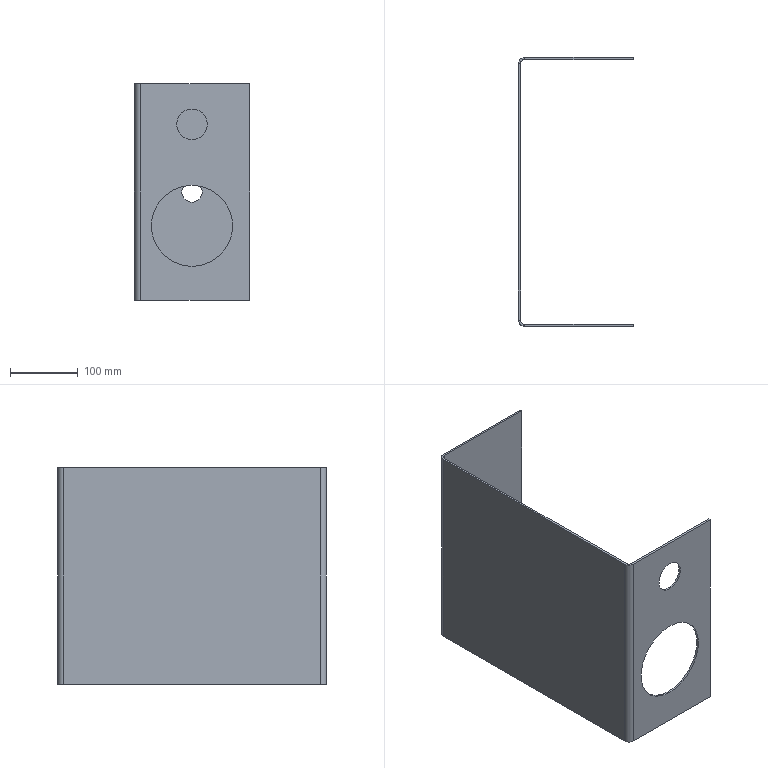Part | SolidWorks | features Cut 2, FlatPattern 1, SMBaseFlange 1, SheetMetal 1 | 1 solid | 28 faces | box 170 x 397 x 320 mm | volume 654758 mm3 | plane 18 | cylinder 10 | commonest cylinder face diameters 12 x2 18 x2 30 x2 45 x2 120 x2
STEP:
#1=CARTESIAN_POINT('',(79.,197.5,175.));
#2=VERTEX_POINT('',#1);
#3=CARTESIAN_POINT('',(79.,197.5,145.));
#4=VERTEX_POINT('',#3);
#5=CARTESIAN_POINT('',(79.,197.5,160.));
#6=DIRECTION('',(0.,-1.,0.));
#7=DIRECTION('',(0.,0.,-1.));
#8=AXIS2_PLACEMENT_3D('',#5,#6,#7);
#9=CIRCLE('',#8,15.);
#10=EDGE_CURVE('',#2,#4,#9,.T.);
#11=ORIENTED_EDGE('',*,*,#10,.T.);
#12=CARTESIAN_POINT('',(79.,200.5,145.));
#13=VERTEX_POINT('',#12);
#14=CARTESIAN_POINT('',(79.,190.5,145.));
#15=DIRECTION('',(0.,1.,0.));
#16=VECTOR('',#15,1000.);
#17=LINE('',#14,#16);
#18=EDGE_CURVE('',#4,#13,#17,.T.);
#19=ORIENTED_EDGE('',*,*,#18,.T.);
#20=CARTESIAN_POINT('',(79.,200.5,175.));
#21=VERTEX_POINT('',#20);
#22=CARTESIAN_POINT('',(79.,200.5,160.));
#23=DIRECTION('',(0.,1.,0.));
#24=DIRECTION('',(0.,0.,1.));
#25=AXIS2_PLACEMENT_3D('',#22,#23,#24);
#26=CIRCLE('',#25,15.);
#27=EDGE_CURVE('',#13,#21,#26,.T.);
#28=ORIENTED_EDGE('',*,*,#27,.T.);
#29=CARTESIAN_POINT('',(79.,190.5,175.));
#30=DIRECTION('',(0.,1.,0.));
#31=VECTOR('',#30,1000.);
#32=LINE('',#29,#31);
#33=EDGE_CURVE('',#2,#21,#32,.T.);
#34=ORIENTED_EDGE('',*,*,#33,.F.);
#35=EDGE_LOOP('',(#11,#19,#28,#34));
#36=FACE_OUTER_BOUND('',#35,.T.);
#37=CARTESIAN_POINT('',(79.,190.5,160.));
#38=DIRECTION('',(0.,1.,0.));
#39=DIRECTION('',(0.,0.,1.));
#40=AXIS2_PLACEMENT_3D('',#37,#38,#39);
#41=CYLINDRICAL_SURFACE('',#40,15.);
#42=ADVANCED_FACE('',(#36),#41,.F.);
#43=CARTESIAN_POINT('',(79.,-193.5,50.));
#44=VERTEX_POINT('',#43);
#45=CARTESIAN_POINT('',(79.,-193.5,170.));
#46=VERTEX_POINT('',#45);
#47=CARTESIAN_POINT('',(79.,-193.5,110.));
#48=DIRECTION('',(0.,1.,0.));
#49=DIRECTION('',(0.,0.,1.));
#50=AXIS2_PLACEMENT_3D('',#47,#48,#49);
#51=CIRCLE('',#50,60.);
#52=EDGE_CURVE('',#44,#46,#51,.T.);
#53=ORIENTED_EDGE('',*,*,#52,.T.);
#54=CARTESIAN_POINT('',(79.,-196.5,170.));
#55=VERTEX_POINT('',#54);
#56=CARTESIAN_POINT('',(79.,-186.5,170.));
#57=DIRECTION('',(0.,-1.,0.));
#58=VECTOR('',#57,1000.);
#59=LINE('',#56,#58);
#60=EDGE_CURVE('',#46,#55,#59,.T.);
#61=ORIENTED_EDGE('',*,*,#60,.T.);
#62=CARTESIAN_POINT('',(79.,-196.5,50.));
#63=VERTEX_POINT('',#62);
#64=CARTESIAN_POINT('',(79.,-196.5,110.));
#65=DIRECTION('',(0.,-1.,0.));
#66=DIRECTION('',(0.,0.,1.));
#67=AXIS2_PLACEMENT_3D('',#64,#65,#66);
#68=CIRCLE('',#67,60.);
#69=EDGE_CURVE('',#55,#63,#68,.T.);
#70=ORIENTED_EDGE('',*,*,#69,.T.);
#71=CARTESIAN_POINT('',(79.,-186.5,50.));
#72=DIRECTION('',(0.,-1.,0.));
#73=VECTOR('',#72,1000.);
#74=LINE('',#71,#73);
#75=EDGE_CURVE('',#44,#63,#74,.T.);
#76=ORIENTED_EDGE('',*,*,#75,.F.);
#77=EDGE_LOOP('',(#53,#61,#70,#76));
#78=FACE_OUTER_BOUND('',#77,.T.);
#79=CARTESIAN_POINT('',(79.,-186.5,110.));
#80=DIRECTION('',(0.,-1.,0.));
#81=DIRECTION('',(0.,0.,-1.));
#82=AXIS2_PLACEMENT_3D('',#79,#80,#81);
#83=CYLINDRICAL_SURFACE('',#82,60.);
#84=ADVANCED_FACE('',(#78),#83,.F.);
#85=CARTESIAN_POINT('',(79.,-193.5,237.5));
#86=VERTEX_POINT('',#85);
#87=CARTESIAN_POINT('',(79.,-193.5,282.5));
#88=VERTEX_POINT('',#87);
#89=CARTESIAN_POINT('',(79.,-193.5,260.));
#90=DIRECTION('',(0.,1.,0.));
#91=DIRECTION('',(0.,0.,1.));
#92=AXIS2_PLACEMENT_3D('',#89,#90,#91);
#93=CIRCLE('',#92,22.5);
#94=EDGE_CURVE('',#86,#88,#93,.T.);
#95=ORIENTED_EDGE('',*,*,#94,.T.);
#96=CARTESIAN_POINT('',(79.,-196.5,282.5));
#97=VERTEX_POINT('',#96);
#98=CARTESIAN_POINT('',(79.,-186.5,282.5));
#99=DIRECTION('',(0.,-1.,0.));
#100=VECTOR('',#99,1000.);
#101=LINE('',#98,#100);
#102=EDGE_CURVE('',#88,#97,#101,.T.);
#103=ORIENTED_EDGE('',*,*,#102,.T.);
#104=CARTESIAN_POINT('',(79.,-196.5,237.5));
#105=VERTEX_POINT('',#104);
#106=CARTESIAN_POINT('',(79.,-196.5,260.));
#107=DIRECTION('',(0.,-1.,0.));
#108=DIRECTION('',(0.,0.,1.));
#109=AXIS2_PLACEMENT_3D('',#106,#107,#108);
#110=CIRCLE('',#109,22.5);
#111=EDGE_CURVE('',#97,#105,#110,.T.);
#112=ORIENTED_EDGE('',*,*,#111,.T.);
#113=CARTESIAN_POINT('',(79.,-186.5,237.5));
#114=DIRECTION('',(0.,-1.,0.));
#115=VECTOR('',#114,1000.);
#116=LINE('',#113,#115);
#117=EDGE_CURVE('',#86,#105,#116,.T.);
#118=ORIENTED_EDGE('',*,*,#117,.F.);
#119=EDGE_LOOP('',(#95,#103,#112,#118));
#120=FACE_OUTER_BOUND('',#119,.T.);
#121=CARTESIAN_POINT('',(79.,-186.5,260.));
#122=DIRECTION('',(0.,-1.,0.));
#123=DIRECTION('',(0.,0.,-1.));
#124=AXIS2_PLACEMENT_3D('',#121,#122,#123);
#125=CYLINDRICAL_SURFACE('',#124,22.5);
#126=ADVANCED_FACE('',(#120),#125,.F.);
#127=CARTESIAN_POINT('',(-3.,191.5,320.));
#128=VERTEX_POINT('',#127);
#129=CARTESIAN_POINT('',(-6.,191.5,320.));
#130=VERTEX_POINT('',#129);
#131=CARTESIAN_POINT('',(-3.,191.5,320.));
#132=DIRECTION('',(-1.,0.,0.));
#133=VECTOR('',#132,1000.);
#134=LINE('',#131,#133);
#135=EDGE_CURVE('',#128,#130,#134,.T.);
#136=ORIENTED_EDGE('',*,*,#135,.F.);
#137=CARTESIAN_POINT('',(3.,197.5,320.));
#138=VERTEX_POINT('',#137);
#139=CARTESIAN_POINT('',(3.,191.5,320.));
#140=DIRECTION('',(0.,0.,1.));
#141=DIRECTION('',(-1.,0.,0.));
#142=AXIS2_PLACEMENT_3D('',#139,#140,#141);
#143=CIRCLE('',#142,6.);
#144=EDGE_CURVE('',#138,#128,#143,.T.);
#145=ORIENTED_EDGE('',*,*,#144,.F.);
#146=CARTESIAN_POINT('',(3.,200.5,320.));
#147=VERTEX_POINT('',#146);
#148=CARTESIAN_POINT('',(3.,200.5,320.));
#149=DIRECTION('',(0.,-1.,0.));
#150=VECTOR('',#149,1000.);
#151=LINE('',#148,#150);
#152=EDGE_CURVE('',#147,#138,#151,.T.);
#153=ORIENTED_EDGE('',*,*,#152,.F.);
#154=CARTESIAN_POINT('',(3.,191.5,320.));
#155=DIRECTION('',(0.,0.,1.));
#156=DIRECTION('',(1.,0.,0.));
#157=AXIS2_PLACEMENT_3D('',#154,#155,#156);
#158=CIRCLE('',#157,9.);
#159=EDGE_CURVE('',#147,#130,#158,.T.);
#160=ORIENTED_EDGE('',*,*,#159,.T.);
#161=EDGE_LOOP('',(#136,#145,#153,#160));
#162=FACE_OUTER_BOUND('',#161,.T.);
#163=CARTESIAN_POINT('',(-3.,191.5,320.));
#164=DIRECTION('',(0.,0.,1.));
#165=DIRECTION('',(1.,0.,0.));
#166=AXIS2_PLACEMENT_3D('',#163,#164,#165);
#167=PLANE('',#166);
#168=ADVANCED_FACE('',(#162),#167,.T.);
#169=CARTESIAN_POINT('',(-3.,-187.5,320.));
#170=VERTEX_POINT('',#169);
#171=CARTESIAN_POINT('',(-3.,-187.5,320.));
#172=DIRECTION('',(0.,-1.,0.));
#173=VECTOR('',#172,1000.);
#174=LINE('',#171,#173);
#175=EDGE_CURVE('',#128,#170,#174,.T.);
#176=ORIENTED_EDGE('',*,*,#175,.F.);
#177=ORIENTED_EDGE('',*,*,#135,.T.);
#178=CARTESIAN_POINT('',(-6.,-187.5,320.));
#179=VERTEX_POINT('',#178);
#180=CARTESIAN_POINT('',(-6.,-187.5,320.));
#181=DIRECTION('',(0.,-1.,0.));
#182=VECTOR('',#181,1000.);
#183=LINE('',#180,#182);
#184=EDGE_CURVE('',#130,#179,#183,.T.);
#185=ORIENTED_EDGE('',*,*,#184,.T.);
#186=CARTESIAN_POINT('',(-6.,-187.5,320.));
#187=DIRECTION('',(1.,0.,0.));
#188=VECTOR('',#187,1000.);
#189=LINE('',#186,#188);
#190=EDGE_CURVE('',#179,#170,#189,.T.);
#191=ORIENTED_EDGE('',*,*,#190,.T.);
#192=EDGE_LOOP('',(#176,#177,#185,#191));
#193=FACE_OUTER_BOUND('',#192,.T.);
#194=CARTESIAN_POINT('',(3.,200.5,320.));
#195=DIRECTION('',(0.,0.,1.));
#196=DIRECTION('',(1.,0.,0.));
#197=AXIS2_PLACEMENT_3D('',#194,#195,#196);
#198=PLANE('',#197);
#199=ADVANCED_FACE('',(#193),#198,.T.);
#200=CARTESIAN_POINT('',(3.,197.5,0.));
#201=VERTEX_POINT('',#200);
#202=CARTESIAN_POINT('',(3.,200.5,0.));
#203=VERTEX_POINT('',#202);
#204=CARTESIAN_POINT('',(3.,197.5,0.));
#205=DIRECTION('',(0.,1.,0.));
#206=VECTOR('',#205,1000.);
#207=LINE('',#204,#206);
#208=EDGE_CURVE('',#201,#203,#207,.T.);
#209=ORIENTED_EDGE('',*,*,#208,.F.);
#210=CARTESIAN_POINT('',(-3.,191.5,0.));
#211=VERTEX_POINT('',#210);
#212=CARTESIAN_POINT('',(3.,191.5,0.));
#213=DIRECTION('',(0.,0.,1.));
#214=DIRECTION('',(-1.,0.,0.));
#215=AXIS2_PLACEMENT_3D('',#212,#213,#214);
#216=CIRCLE('',#215,6.);
#217=EDGE_CURVE('',#201,#211,#216,.T.);
#218=ORIENTED_EDGE('',*,*,#217,.T.);
#219=CARTESIAN_POINT('',(-6.,191.5,0.));
#220=VERTEX_POINT('',#219);
#221=CARTESIAN_POINT('',(-6.,191.5,0.));
#222=DIRECTION('',(1.,0.,0.));
#223=VECTOR('',#222,1000.);
#224=LINE('',#221,#223);
#225=EDGE_CURVE('',#220,#211,#224,.T.);
#226=ORIENTED_EDGE('',*,*,#225,.F.);
#227=CARTESIAN_POINT('',(3.,191.5,0.));
#228=DIRECTION('',(0.,0.,1.));
#229=DIRECTION('',(1.,0.,0.));
#230=AXIS2_PLACEMENT_3D('',#227,#228,#229);
#231=CIRCLE('',#230,9.);
#232=EDGE_CURVE('',#203,#220,#231,.T.);
#233=ORIENTED_EDGE('',*,*,#232,.F.);
#234=EDGE_LOOP('',(#209,#218,#226,#233));
#235=FACE_OUTER_BOUND('',#234,.T.);
#236=CARTESIAN_POINT('',(3.,197.5,0.));
#237=DIRECTION('',(0.,0.,-1.));
#238=DIRECTION('',(-1.,0.,0.));
#239=AXIS2_PLACEMENT_3D('',#236,#237,#238);
#240=PLANE('',#239);
#241=ADVANCED_FACE('',(#235),#240,.T.);
#242=CARTESIAN_POINT('',(164.,197.5,0.));
#243=VERTEX_POINT('',#242);
#244=CARTESIAN_POINT('',(3.,197.5,0.));
#245=DIRECTION('',(-1.,0.,0.));
#246=VECTOR('',#245,1000.);
#247=LINE('',#244,#246);
#248=EDGE_CURVE('',#243,#201,#247,.T.);
#249=ORIENTED_EDGE('',*,*,#248,.T.);
#250=ORIENTED_EDGE('',*,*,#208,.T.);
#251=CARTESIAN_POINT('',(164.,200.5,0.));
#252=VERTEX_POINT('',#251);
#253=CARTESIAN_POINT('',(3.,200.5,0.));
#254=DIRECTION('',(-1.,0.,0.));
#255=VECTOR('',#254,1000.);
#256=LINE('',#253,#255);
#257=EDGE_CURVE('',#252,#203,#256,.T.);
#258=ORIENTED_EDGE('',*,*,#257,.F.);
#259=CARTESIAN_POINT('',(164.,200.5,0.));
#260=DIRECTION('',(0.,-1.,0.));
#261=VECTOR('',#260,1000.);
#262=LINE('',#259,#261);
#263=EDGE_CURVE('',#252,#243,#262,.T.);
#264=ORIENTED_EDGE('',*,*,#263,.T.);
#265=EDGE_LOOP('',(#249,#250,#258,#264));
#266=FACE_OUTER_BOUND('',#265,.T.);
#267=CARTESIAN_POINT('',(-6.,191.5,0.));
#268=DIRECTION('',(0.,0.,-1.));
#269=DIRECTION('',(-1.,0.,0.));
#270=AXIS2_PLACEMENT_3D('',#267,#268,#269);
#271=PLANE('',#270);
#272=ADVANCED_FACE('',(#266),#271,.T.);
#273=CARTESIAN_POINT('',(3.,-193.5,320.));
#274=VERTEX_POINT('',#273);
#275=CARTESIAN_POINT('',(3.,-196.5,320.));
#276=VERTEX_POINT('',#275);
#277=CARTESIAN_POINT('',(3.,-193.5,320.));
#278=DIRECTION('',(0.,-1.,0.));
#279=VECTOR('',#278,1000.);
#280=LINE('',#277,#279);
#281=EDGE_CURVE('',#274,#276,#280,.T.);
#282=ORIENTED_EDGE('',*,*,#281,.F.);
#283=CARTESIAN_POINT('',(3.,-187.5,320.));
#284=DIRECTION('',(0.,0.,1.));
#285=DIRECTION('',(1.,0.,0.));
#286=AXIS2_PLACEMENT_3D('',#283,#284,#285);
#287=CIRCLE('',#286,6.);
#288=EDGE_CURVE('',#170,#274,#287,.T.);
#289=ORIENTED_EDGE('',*,*,#288,.F.);
#290=ORIENTED_EDGE('',*,*,#190,.F.);
#291=CARTESIAN_POINT('',(3.,-187.5,320.));
#292=DIRECTION('',(0.,0.,1.));
#293=DIRECTION('',(1.,0.,0.));
#294=AXIS2_PLACEMENT_3D('',#291,#292,#293);
#295=CIRCLE('',#294,9.);
#296=EDGE_CURVE('',#179,#276,#295,.T.);
#297=ORIENTED_EDGE('',*,*,#296,.T.);
#298=EDGE_LOOP('',(#282,#289,#290,#297));
#299=FACE_OUTER_BOUND('',#298,.T.);
#300=CARTESIAN_POINT('',(3.,-193.5,320.));
#301=DIRECTION('',(0.,0.,1.));
#302=DIRECTION('',(1.,0.,0.));
#303=AXIS2_PLACEMENT_3D('',#300,#301,#302);
#304=PLANE('',#303);
#305=ADVANCED_FACE('',(#299),#304,.T.);
#306=CARTESIAN_POINT('',(164.,-193.5,320.));
#307=VERTEX_POINT('',#306);
#308=CARTESIAN_POINT('',(3.,-193.5,320.));
#309=DIRECTION('',(1.,0.,0.));
#310=VECTOR('',#309,1000.);
#311=LINE('',#308,#310);
#312=EDGE_CURVE('',#274,#307,#311,.T.);
#313=ORIENTED_EDGE('',*,*,#312,.F.);
#314=ORIENTED_EDGE('',*,*,#281,.T.);
#315=CARTESIAN_POINT('',(164.,-196.5,320.));
#316=VERTEX_POINT('',#315);
#317=CARTESIAN_POINT('',(3.,-196.5,320.));
#318=DIRECTION('',(1.,0.,0.));
#319=VECTOR('',#318,1000.);
#320=LINE('',#317,#319);
#321=EDGE_CURVE('',#276,#316,#320,.T.);
#322=ORIENTED_EDGE('',*,*,#321,.T.);
#323=CARTESIAN_POINT('',(164.,-193.5,320.));
#324=DIRECTION('',(0.,-1.,0.));
#325=VECTOR('',#324,1000.);
#326=LINE('',#323,#325);
#327=EDGE_CURVE('',#307,#316,#326,.T.);
#328=ORIENTED_EDGE('',*,*,#327,.F.);
#329=EDGE_LOOP('',(#313,#314,#322,#328));
#330=FACE_OUTER_BOUND('',#329,.T.);
#331=CARTESIAN_POINT('',(-6.,-187.5,320.));
#332=DIRECTION('',(0.,0.,1.));
#333=DIRECTION('',(1.,0.,0.));
#334=AXIS2_PLACEMENT_3D('',#331,#332,#333);
#335=PLANE('',#334);
#336=ADVANCED_FACE('',(#330),#335,.T.);
#337=CARTESIAN_POINT('',(-3.,-187.5,0.));
#338=VERTEX_POINT('',#337);
#339=CARTESIAN_POINT('',(-6.,-187.5,0.));
#340=VERTEX_POINT('',#339);
#341=CARTESIAN_POINT('',(-3.,-187.5,0.));
#342=DIRECTION('',(-1.,0.,0.));
#343=VECTOR('',#342,1000.);
#344=LINE('',#341,#343);
#345=EDGE_CURVE('',#338,#340,#344,.T.);
#346=ORIENTED_EDGE('',*,*,#345,.F.);
#347=CARTESIAN_POINT('',(3.,-193.5,0.));
#348=VERTEX_POINT('',#347);
#349=CARTESIAN_POINT('',(3.,-187.5,0.));
#350=DIRECTION('',(0.,0.,1.));
#351=DIRECTION('',(1.,0.,0.));
#352=AXIS2_PLACEMENT_3D('',#349,#350,#351);
#353=CIRCLE('',#352,6.);
#354=EDGE_CURVE('',#338,#348,#353,.T.);
#355=ORIENTED_EDGE('',*,*,#354,.T.);
#356=CARTESIAN_POINT('',(3.,-196.5,0.));
#357=VERTEX_POINT('',#356);
#358=CARTESIAN_POINT('',(3.,-196.5,0.));
#359=DIRECTION('',(0.,1.,0.));
#360=VECTOR('',#359,1000.);
#361=LINE('',#358,#360);
#362=EDGE_CURVE('',#357,#348,#361,.T.);
#363=ORIENTED_EDGE('',*,*,#362,.F.);
#364=CARTESIAN_POINT('',(3.,-187.5,0.));
#365=DIRECTION('',(0.,0.,1.));
#366=DIRECTION('',(1.,0.,0.));
#367=AXIS2_PLACEMENT_3D('',#364,#365,#366);
#368=CIRCLE('',#367,9.);
#369=EDGE_CURVE('',#340,#357,#368,.T.);
#370=ORIENTED_EDGE('',*,*,#369,.F.);
#371=EDGE_LOOP('',(#346,#355,#363,#370));
#372=FACE_OUTER_BOUND('',#371,.T.);
#373=CARTESIAN_POINT('',(-3.,-187.5,0.));
#374=DIRECTION('',(0.,0.,-1.));
#375=DIRECTION('',(-1.,0.,0.));
#376=AXIS2_PLACEMENT_3D('',#373,#374,#375);
#377=PLANE('',#376);
#378=ADVANCED_FACE('',(#372),#377,.T.);
#379=CARTESIAN_POINT('',(-3.,-187.5,0.));
#380=DIRECTION('',(0.,-1.,0.));
#381=VECTOR('',#380,1000.);
#382=LINE('',#379,#381);
#383=EDGE_CURVE('',#211,#338,#382,.T.);
#384=ORIENTED_EDGE('',*,*,#383,.T.);
#385=ORIENTED_EDGE('',*,*,#345,.T.);
#386=CARTESIAN_POINT('',(-6.,-187.5,0.));
#387=DIRECTION('',(0.,-1.,0.));
#388=VECTOR('',#387,1000.);
#389=LINE('',#386,#388);
#390=EDGE_CURVE('',#220,#340,#389,.T.);
#391=ORIENTED_EDGE('',*,*,#390,.F.);
#392=ORIENTED_EDGE('',*,*,#225,.T.);
#393=EDGE_LOOP('',(#384,#385,#391,#392));
#394=FACE_OUTER_BOUND('',#393,.T.);
#395=CARTESIAN_POINT('',(3.,-196.5,0.));
#396=DIRECTION('',(0.,0.,-1.));
#397=DIRECTION('',(-1.,0.,0.));
#398=AXIS2_PLACEMENT_3D('',#395,#396,#397);
#399=PLANE('',#398);
#400=ADVANCED_FACE('',(#394),#399,.T.);
#401=CARTESIAN_POINT('',(79.,-196.5,110.));
#402=DIRECTION('',(0.,-1.,0.));
#403=DIRECTION('',(0.,0.,1.));
#404=AXIS2_PLACEMENT_3D('',#401,#402,#403);
#405=CIRCLE('',#404,60.);
#406=EDGE_CURVE('',#63,#55,#405,.T.);
#407=ORIENTED_EDGE('',*,*,#406,.F.);
#408=ORIENTED_EDGE('',*,*,#69,.F.);
#409=EDGE_LOOP('',(#407,#408));
#410=FACE_BOUND('',#409,.T.);
#411=CARTESIAN_POINT('',(79.,-196.5,260.));
#412=DIRECTION('',(0.,-1.,0.));
#413=DIRECTION('',(0.,0.,1.));
#414=AXIS2_PLACEMENT_3D('',#411,#412,#413);
#415=CIRCLE('',#414,22.5);
#416=EDGE_CURVE('',#105,#97,#415,.T.);
#417=ORIENTED_EDGE('',*,*,#416,.F.);
#418=ORIENTED_EDGE('',*,*,#111,.F.);
#419=EDGE_LOOP('',(#417,#418));
#420=FACE_BOUND('',#419,.T.);
#421=CARTESIAN_POINT('',(164.,-196.5,0.));
#422=VERTEX_POINT('',#421);
#423=CARTESIAN_POINT('',(3.,-196.5,0.));
#424=DIRECTION('',(1.,0.,0.));
#425=VECTOR('',#424,1000.);
#426=LINE('',#423,#425);
#427=EDGE_CURVE('',#357,#422,#426,.T.);
#428=ORIENTED_EDGE('',*,*,#427,.T.);
#429=CARTESIAN_POINT('',(164.,-196.5,320.));
#430=DIRECTION('',(0.,0.,-1.));
#431=VECTOR('',#430,1000.);
#432=LINE('',#429,#431);
#433=EDGE_CURVE('',#316,#422,#432,.T.);
#434=ORIENTED_EDGE('',*,*,#433,.F.);
#435=ORIENTED_EDGE('',*,*,#321,.F.);
#436=CARTESIAN_POINT('',(3.,-196.5,320.));
#437=DIRECTION('',(0.,0.,-1.));
#438=VECTOR('',#437,1000.);
#439=LINE('',#436,#438);
#440=EDGE_CURVE('',#276,#357,#439,.T.);
#441=ORIENTED_EDGE('',*,*,#440,.T.);
#442=EDGE_LOOP('',(#428,#434,#435,#441));
#443=FACE_OUTER_BOUND('',#442,.T.);
#444=CARTESIAN_POINT('',(3.,-196.5,320.));
#445=DIRECTION('',(0.,1.,0.));
#446=DIRECTION('',(0.,0.,1.));
#447=AXIS2_PLACEMENT_3D('',#444,#445,#446);
#448=PLANE('',#447);
#449=ADVANCED_FACE('',(#410,#420,#443),#448,.F.);
#450=CARTESIAN_POINT('',(164.,-193.5,0.));
#451=VERTEX_POINT('',#450);
#452=CARTESIAN_POINT('',(164.,-193.5,0.));
#453=DIRECTION('',(0.,-1.,0.));
#454=VECTOR('',#453,1000.);
#455=LINE('',#452,#454);
#456=EDGE_CURVE('',#451,#422,#455,.T.);
#457=ORIENTED_EDGE('',*,*,#456,.F.);
#458=CARTESIAN_POINT('',(164.,-193.5,320.));
#459=DIRECTION('',(0.,0.,-1.));
#460=VECTOR('',#459,1000.);
#461=LINE('',#458,#460);
#462=EDGE_CURVE('',#307,#451,#461,.T.);
#463=ORIENTED_EDGE('',*,*,#462,.F.);
#464=ORIENTED_EDGE('',*,*,#327,.T.);
#465=ORIENTED_EDGE('',*,*,#433,.T.);
#466=EDGE_LOOP('',(#457,#463,#464,#465));
#467=FACE_OUTER_BOUND('',#466,.T.);
#468=CARTESIAN_POINT('',(164.,-193.5,320.));
#469=DIRECTION('',(1.,0.,0.));
#470=DIRECTION('',(0.,0.,-1.));
#471=AXIS2_PLACEMENT_3D('',#468,#469,#470);
#472=PLANE('',#471);
#473=ADVANCED_FACE('',(#467),#472,.T.);
#474=ORIENTED_EDGE('',*,*,#52,.F.);
#475=CARTESIAN_POINT('',(79.,-193.5,110.));
#476=DIRECTION('',(0.,1.,0.));
#477=DIRECTION('',(0.,0.,1.));
#478=AXIS2_PLACEMENT_3D('',#475,#476,#477);
#479=CIRCLE('',#478,60.);
#480=EDGE_CURVE('',#46,#44,#479,.T.);
#481=ORIENTED_EDGE('',*,*,#480,.F.);
#482=EDGE_LOOP('',(#474,#481));
#483=FACE_BOUND('',#482,.T.);
#484=ORIENTED_EDGE('',*,*,#94,.F.);
#485=CARTESIAN_POINT('',(79.,-193.5,260.));
#486=DIRECTION('',(0.,1.,0.));
#487=DIRECTION('',(0.,0.,1.));
#488=AXIS2_PLACEMENT_3D('',#485,#486,#487);
#489=CIRCLE('',#488,22.5);
#490=EDGE_CURVE('',#88,#86,#489,.T.);
#491=ORIENTED_EDGE('',*,*,#490,.F.);
#492=EDGE_LOOP('',(#484,#491));
#493=FACE_BOUND('',#492,.T.);
#494=CARTESIAN_POINT('',(3.,-193.5,0.));
#495=DIRECTION('',(1.,0.,0.));
#496=VECTOR('',#495,1000.);
#497=LINE('',#494,#496);
#498=EDGE_CURVE('',#348,#451,#497,.T.);
#499=ORIENTED_EDGE('',*,*,#498,.F.);
#500=CARTESIAN_POINT('',(3.,-193.5,320.));
#501=DIRECTION('',(0.,0.,-1.));
#502=VECTOR('',#501,1000.);
#503=LINE('',#500,#502);
#504=EDGE_CURVE('',#274,#348,#503,.T.);
#505=ORIENTED_EDGE('',*,*,#504,.F.);
#506=ORIENTED_EDGE('',*,*,#312,.T.);
#507=ORIENTED_EDGE('',*,*,#462,.T.);
#508=EDGE_LOOP('',(#499,#505,#506,#507));
#509=FACE_OUTER_BOUND('',#508,.T.);
#510=CARTESIAN_POINT('',(3.,-193.5,320.));
#511=DIRECTION('',(0.,1.,0.));
#512=DIRECTION('',(0.,0.,1.));
#513=AXIS2_PLACEMENT_3D('',#510,#511,#512);
#514=PLANE('',#513);
#515=ADVANCED_FACE('',(#483,#493,#509),#514,.T.);
#516=ORIENTED_EDGE('',*,*,#354,.F.);
#517=CARTESIAN_POINT('',(-3.,-187.5,320.));
#518=DIRECTION('',(0.,0.,-1.));
#519=VECTOR('',#518,1000.);
#520=LINE('',#517,#519);
#521=EDGE_CURVE('',#170,#338,#520,.T.);
#522=ORIENTED_EDGE('',*,*,#521,.F.);
#523=ORIENTED_EDGE('',*,*,#288,.T.);
#524=ORIENTED_EDGE('',*,*,#504,.T.);
#525=EDGE_LOOP('',(#516,#522,#523,#524));
#526=FACE_OUTER_BOUND('',#525,.T.);
#527=CARTESIAN_POINT('',(3.,-187.5,320.));
#528=DIRECTION('',(0.,0.,-1.));
#529=DIRECTION('',(-1.,0.,0.));
#530=AXIS2_PLACEMENT_3D('',#527,#528,#529);
#531=CYLINDRICAL_SURFACE('',#530,6.);
#532=ADVANCED_FACE('',(#526),#531,.F.);
#533=ORIENTED_EDGE('',*,*,#383,.F.);
#534=CARTESIAN_POINT('',(-3.,191.5,320.));
#535=DIRECTION('',(0.,0.,-1.));
#536=VECTOR('',#535,1000.);
#537=LINE('',#534,#536);
#538=EDGE_CURVE('',#128,#211,#537,.T.);
#539=ORIENTED_EDGE('',*,*,#538,.F.);
#540=ORIENTED_EDGE('',*,*,#175,.T.);
#541=ORIENTED_EDGE('',*,*,#521,.T.);
#542=EDGE_LOOP('',(#533,#539,#540,#541));
#543=FACE_OUTER_BOUND('',#542,.T.);
#544=CARTESIAN_POINT('',(-3.,-187.5,320.));
#545=DIRECTION('',(1.,0.,0.));
#546=DIRECTION('',(0.,0.,-1.));
#547=AXIS2_PLACEMENT_3D('',#544,#545,#546);
#548=PLANE('',#547);
#549=ADVANCED_FACE('',(#543),#548,.T.);
#550=ORIENTED_EDGE('',*,*,#217,.F.);
#551=CARTESIAN_POINT('',(3.,197.5,320.));
#552=DIRECTION('',(0.,0.,-1.));
#553=VECTOR('',#552,1000.);
#554=LINE('',#551,#553);
#555=EDGE_CURVE('',#138,#201,#554,.T.);
#556=ORIENTED_EDGE('',*,*,#555,.F.);
#557=ORIENTED_EDGE('',*,*,#144,.T.);
#558=ORIENTED_EDGE('',*,*,#538,.T.);
#559=EDGE_LOOP('',(#550,#556,#557,#558));
#560=FACE_OUTER_BOUND('',#559,.T.);
#561=CARTESIAN_POINT('',(3.,191.5,320.));
#562=DIRECTION('',(0.,0.,-1.));
#563=DIRECTION('',(-1.,0.,0.));
#564=AXIS2_PLACEMENT_3D('',#561,#562,#563);
#565=CYLINDRICAL_SURFACE('',#564,6.);
#566=ADVANCED_FACE('',(#560),#565,.F.);
#567=ORIENTED_EDGE('',*,*,#10,.F.);
#568=CARTESIAN_POINT('',(79.,197.5,160.));
#569=DIRECTION('',(0.,-1.,0.));
#570=DIRECTION('',(0.,0.,-1.));
#571=AXIS2_PLACEMENT_3D('',#568,#569,#570);
#572=CIRCLE('',#571,15.);
#573=EDGE_CURVE('',#4,#2,#572,.T.);
#574=ORIENTED_EDGE('',*,*,#573,.F.);
#575=EDGE_LOOP('',(#567,#574));
#576=FACE_BOUND('',#575,.T.);
#577=ORIENTED_EDGE('',*,*,#248,.F.);
#578=CARTESIAN_POINT('',(164.,197.5,320.));
#579=VERTEX_POINT('',#578);
#580=CARTESIAN_POINT('',(164.,197.5,320.));
#581=DIRECTION('',(0.,0.,-1.));
#582=VECTOR('',#581,1000.);
#583=LINE('',#580,#582);
#584=EDGE_CURVE('',#579,#243,#583,.T.);
#585=ORIENTED_EDGE('',*,*,#584,.F.);
#586=CARTESIAN_POINT('',(3.,197.5,320.));
#587=DIRECTION('',(-1.,0.,0.));
#588=VECTOR('',#587,1000.);
#589=LINE('',#586,#588);
#590=EDGE_CURVE('',#579,#138,#589,.T.);
#591=ORIENTED_EDGE('',*,*,#590,.T.);
#592=ORIENTED_EDGE('',*,*,#555,.T.);
#593=EDGE_LOOP('',(#577,#585,#591,#592));
#594=FACE_OUTER_BOUND('',#593,.T.);
#595=CARTESIAN_POINT('',(3.,197.5,320.));
#596=DIRECTION('',(0.,-1.,0.));
#597=DIRECTION('',(0.,0.,-1.));
#598=AXIS2_PLACEMENT_3D('',#595,#596,#597);
#599=PLANE('',#598);
#600=ADVANCED_FACE('',(#576,#594),#599,.T.);
#601=ORIENTED_EDGE('',*,*,#263,.F.);
#602=CARTESIAN_POINT('',(164.,200.5,320.));
#603=VERTEX_POINT('',#602);
#604=CARTESIAN_POINT('',(164.,200.5,320.));
#605=DIRECTION('',(0.,0.,-1.));
#606=VECTOR('',#605,1000.);
#607=LINE('',#604,#606);
#608=EDGE_CURVE('',#603,#252,#607,.T.);
#609=ORIENTED_EDGE('',*,*,#608,.F.);
#610=CARTESIAN_POINT('',(164.,200.5,320.));
#611=DIRECTION('',(0.,-1.,0.));
#612=VECTOR('',#611,1000.);
#613=LINE('',#610,#612);
#614=EDGE_CURVE('',#603,#579,#613,.T.);
#615=ORIENTED_EDGE('',*,*,#614,.T.);
#616=ORIENTED_EDGE('',*,*,#584,.T.);
#617=EDGE_LOOP('',(#601,#609,#615,#616));
#618=FACE_OUTER_BOUND('',#617,.T.);
#619=CARTESIAN_POINT('',(164.,200.5,320.));
#620=DIRECTION('',(1.,0.,0.));
#621=DIRECTION('',(0.,0.,-1.));
#622=AXIS2_PLACEMENT_3D('',#619,#620,#621);
#623=PLANE('',#622);
#624=ADVANCED_FACE('',(#618),#623,.T.);
#625=CARTESIAN_POINT('',(79.,200.5,160.));
#626=DIRECTION('',(0.,1.,0.));
#627=DIRECTION('',(0.,0.,1.));
#628=AXIS2_PLACEMENT_3D('',#625,#626,#627);
#629=CIRCLE('',#628,15.);
#630=EDGE_CURVE('',#21,#13,#629,.T.);
#631=ORIENTED_EDGE('',*,*,#630,.F.);
#632=ORIENTED_EDGE('',*,*,#27,.F.);
#633=EDGE_LOOP('',(#631,#632));
#634=FACE_BOUND('',#633,.T.);
#635=ORIENTED_EDGE('',*,*,#257,.T.);
#636=CARTESIAN_POINT('',(3.,200.5,320.));
#637=DIRECTION('',(0.,0.,-1.));
#638=VECTOR('',#637,1000.);
#639=LINE('',#636,#638);
#640=EDGE_CURVE('',#147,#203,#639,.T.);
#641=ORIENTED_EDGE('',*,*,#640,.F.);
#642=CARTESIAN_POINT('',(3.,200.5,320.));
#643=DIRECTION('',(-1.,0.,0.));
#644=VECTOR('',#643,1000.);
#645=LINE('',#642,#644);
#646=EDGE_CURVE('',#603,#147,#645,.T.);
#647=ORIENTED_EDGE('',*,*,#646,.F.);
#648=ORIENTED_EDGE('',*,*,#608,.T.);
#649=EDGE_LOOP('',(#635,#641,#647,#648));
#650=FACE_OUTER_BOUND('',#649,.T.);
#651=CARTESIAN_POINT('',(3.,200.5,320.));
#652=DIRECTION('',(0.,-1.,0.));
#653=DIRECTION('',(0.,0.,-1.));
#654=AXIS2_PLACEMENT_3D('',#651,#652,#653);
#655=PLANE('',#654);
#656=ADVANCED_FACE('',(#634,#650),#655,.F.);
#657=ORIENTED_EDGE('',*,*,#232,.T.);
#658=CARTESIAN_POINT('',(-6.,191.5,320.));
#659=DIRECTION('',(0.,0.,-1.));
#660=VECTOR('',#659,1000.);
#661=LINE('',#658,#660);
#662=EDGE_CURVE('',#130,#220,#661,.T.);
#663=ORIENTED_EDGE('',*,*,#662,.F.);
#664=ORIENTED_EDGE('',*,*,#159,.F.);
#665=ORIENTED_EDGE('',*,*,#640,.T.);
#666=EDGE_LOOP('',(#657,#663,#664,#665));
#667=FACE_OUTER_BOUND('',#666,.T.);
#668=CARTESIAN_POINT('',(3.,191.5,320.));
#669=DIRECTION('',(0.,0.,-1.));
#670=DIRECTION('',(-1.,0.,0.));
#671=AXIS2_PLACEMENT_3D('',#668,#669,#670);
#672=CYLINDRICAL_SURFACE('',#671,9.);
#673=ADVANCED_FACE('',(#667),#672,.T.);
#674=ORIENTED_EDGE('',*,*,#390,.T.);
#675=CARTESIAN_POINT('',(-6.,-187.5,320.));
#676=DIRECTION('',(0.,0.,-1.));
#677=VECTOR('',#676,1000.);
#678=LINE('',#675,#677);
#679=EDGE_CURVE('',#179,#340,#678,.T.);
#680=ORIENTED_EDGE('',*,*,#679,.F.);
#681=ORIENTED_EDGE('',*,*,#184,.F.);
#682=ORIENTED_EDGE('',*,*,#662,.T.);
#683=EDGE_LOOP('',(#674,#680,#681,#682));
#684=FACE_OUTER_BOUND('',#683,.T.);
#685=CARTESIAN_POINT('',(-6.,-187.5,320.));
#686=DIRECTION('',(1.,0.,0.));
#687=DIRECTION('',(0.,0.,-1.));
#688=AXIS2_PLACEMENT_3D('',#685,#686,#687);
#689=PLANE('',#688);
#690=ADVANCED_FACE('',(#684),#689,.F.);
#691=ORIENTED_EDGE('',*,*,#369,.T.);
#692=ORIENTED_EDGE('',*,*,#440,.F.);
#693=ORIENTED_EDGE('',*,*,#296,.F.);
#694=ORIENTED_EDGE('',*,*,#679,.T.);
#695=EDGE_LOOP('',(#691,#692,#693,#694));
#696=FACE_OUTER_BOUND('',#695,.T.);
#697=CARTESIAN_POINT('',(3.,-187.5,320.));
#698=DIRECTION('',(0.,0.,-1.));
#699=DIRECTION('',(-1.,0.,0.));
#700=AXIS2_PLACEMENT_3D('',#697,#698,#699);
#701=CYLINDRICAL_SURFACE('',#700,9.);
#702=ADVANCED_FACE('',(#696),#701,.T.);
#703=ORIENTED_EDGE('',*,*,#646,.T.);
#704=ORIENTED_EDGE('',*,*,#152,.T.);
#705=ORIENTED_EDGE('',*,*,#590,.F.);
#706=ORIENTED_EDGE('',*,*,#614,.F.);
#707=EDGE_LOOP('',(#703,#704,#705,#706));
#708=FACE_OUTER_BOUND('',#707,.T.);
#709=CARTESIAN_POINT('',(3.,-187.5,320.));
#710=DIRECTION('',(0.,0.,1.));
#711=DIRECTION('',(1.,0.,0.));
#712=AXIS2_PLACEMENT_3D('',#709,#710,#711);
#713=PLANE('',#712);
#714=ADVANCED_FACE('',(#708),#713,.T.);
#715=ORIENTED_EDGE('',*,*,#427,.F.);
#716=ORIENTED_EDGE('',*,*,#362,.T.);
#717=ORIENTED_EDGE('',*,*,#498,.T.);
#718=ORIENTED_EDGE('',*,*,#456,.T.);
#719=EDGE_LOOP('',(#715,#716,#717,#718));
#720=FACE_OUTER_BOUND('',#719,.T.);
#721=CARTESIAN_POINT('',(3.,-187.5,0.));
#722=DIRECTION('',(0.,0.,1.));
#723=DIRECTION('',(1.,0.,0.));
#724=AXIS2_PLACEMENT_3D('',#721,#722,#723);
#725=PLANE('',#724);
#726=ADVANCED_FACE('',(#720),#725,.F.);
#727=ORIENTED_EDGE('',*,*,#102,.F.);
#728=ORIENTED_EDGE('',*,*,#490,.T.);
#729=ORIENTED_EDGE('',*,*,#117,.T.);
#730=ORIENTED_EDGE('',*,*,#416,.T.);
#731=EDGE_LOOP('',(#727,#728,#729,#730));
#732=FACE_OUTER_BOUND('',#731,.T.);
#733=CARTESIAN_POINT('',(79.,-186.5,260.));
#734=DIRECTION('',(0.,-1.,0.));
#735=DIRECTION('',(0.,0.,-1.));
#736=AXIS2_PLACEMENT_3D('',#733,#734,#735);
#737=CYLINDRICAL_SURFACE('',#736,22.5);
#738=ADVANCED_FACE('',(#732),#737,.F.);
#739=ORIENTED_EDGE('',*,*,#60,.F.);
#740=ORIENTED_EDGE('',*,*,#480,.T.);
#741=ORIENTED_EDGE('',*,*,#75,.T.);
#742=ORIENTED_EDGE('',*,*,#406,.T.);
#743=EDGE_LOOP('',(#739,#740,#741,#742));
#744=FACE_OUTER_BOUND('',#743,.T.);
#745=CARTESIAN_POINT('',(79.,-186.5,110.));
#746=DIRECTION('',(0.,-1.,0.));
#747=DIRECTION('',(0.,0.,-1.));
#748=AXIS2_PLACEMENT_3D('',#745,#746,#747);
#749=CYLINDRICAL_SURFACE('',#748,60.);
#750=ADVANCED_FACE('',(#744),#749,.F.);
#751=ORIENTED_EDGE('',*,*,#18,.F.);
#752=ORIENTED_EDGE('',*,*,#573,.T.);
#753=ORIENTED_EDGE('',*,*,#33,.T.);
#754=ORIENTED_EDGE('',*,*,#630,.T.);
#755=EDGE_LOOP('',(#751,#752,#753,#754));
#756=FACE_OUTER_BOUND('',#755,.T.);
#757=CARTESIAN_POINT('',(79.,190.5,160.));
#758=DIRECTION('',(0.,1.,0.));
#759=DIRECTION('',(0.,0.,1.));
#760=AXIS2_PLACEMENT_3D('',#757,#758,#759);
#761=CYLINDRICAL_SURFACE('',#760,15.);
#762=ADVANCED_FACE('',(#756),#761,.F.);
#763=CLOSED_SHELL('',(#42,#84,#126,#168,#199,#241,#272,#305,#336,#378,#400,#449,#473,#515,#532,#549,#566,#600,#624,#656,#673,#690,#702,#714,#726,#738,#750,#762));
#764=MANIFOLD_SOLID_BREP('',#763);
#765=CARTESIAN_POINT('',(0.,0.,0.));
#766=DIRECTION('',(0.,0.,1.));
#767=DIRECTION('',(1.,0.,0.));
#768=AXIS2_PLACEMENT_3D('',#765,#766,#767);
#769=(LENGTH_UNIT()NAMED_UNIT(*)SI_UNIT(.MILLI.,.METRE.));
#770=UNCERTAINTY_MEASURE_WITH_UNIT(LENGTH_MEASURE(0.00001),#769,'','');
#771=(NAMED_UNIT(*)PLANE_ANGLE_UNIT()SI_UNIT($,.RADIAN.));
#772=(NAMED_UNIT(*)SI_UNIT($,.STERADIAN.)SOLID_ANGLE_UNIT());
#773=(GEOMETRIC_REPRESENTATION_CONTEXT(3)GLOBAL_UNCERTAINTY_ASSIGNED_CONTEXT((#770))GLOBAL_UNIT_ASSIGNED_CONTEXT((#769,#771,#772))REPRESENTATION_CONTEXT('',''));
#774=ADVANCED_BREP_SHAPE_REPRESENTATION('',(#764,#768),#773);